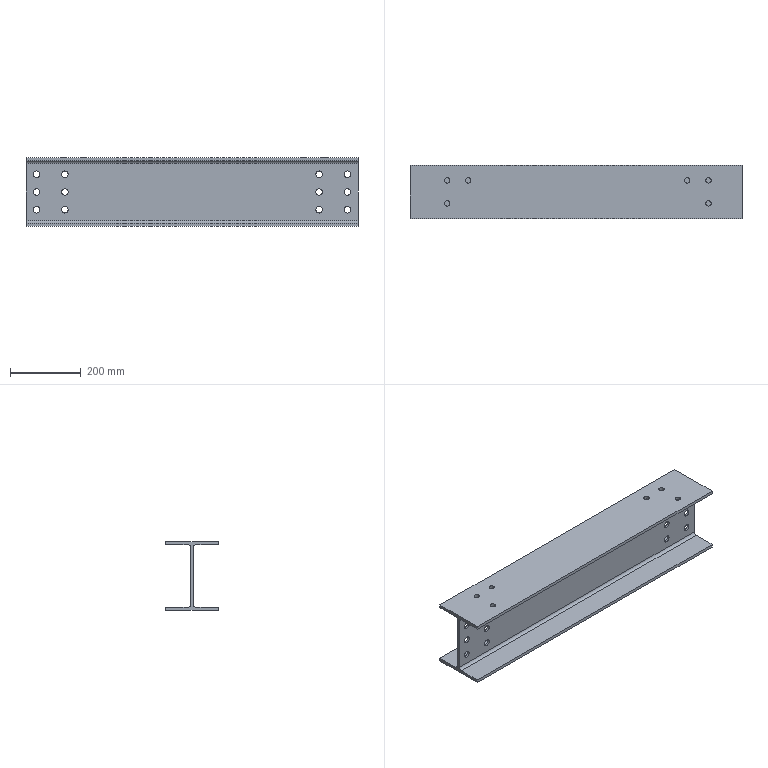Part | STEP file | 粉仓楼梯支承梁主体-194×150_Default<As Machined> | 1 solid | 54 faces | box 940 x 150 x 194 mm | volume 3552325 mm3 | cylinder 40 | plane 14 | commonest cylinder face diameters 19 x24 15 x12 16 x4